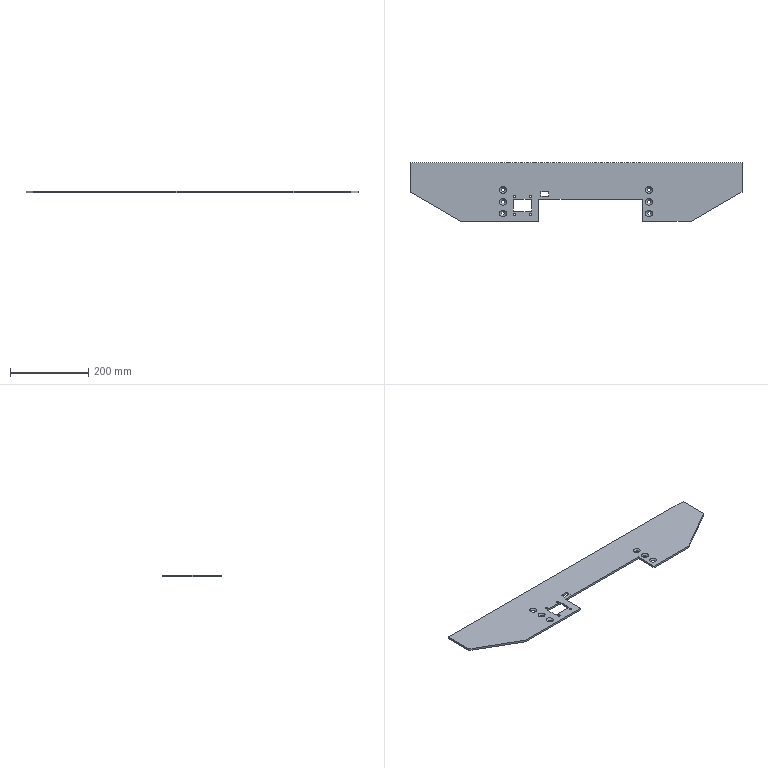Part | NX | features BREP 1 | 1 solid | 40 faces | box 850 x 150 x 5 mm | volume 499921 mm3 | plane 20 | cylinder 14 | cone 6 | commonest cylinder face diameters 9 x6 4 x4 5.2 x4
STEP:
#1=CARTESIAN_POINT('',(-114.45,17.05,0.));
#2=VERTEX_POINT('',#1);
#3=CARTESIAN_POINT('',(-117.05,17.05,0.));
#4=DIRECTION('',(0.,0.,1.));
#5=DIRECTION('',(1.,0.,0.));
#6=AXIS2_PLACEMENT_3D('',#3,#4,#5);
#7=CIRCLE('',#6,2.6);
#8=EDGE_CURVE('',#2,#2,#7,.T.);
#9=ORIENTED_EDGE('',*,*,#8,.T.);
#10=EDGE_LOOP('',(#9));
#11=FACE_BOUND('',#10,.T.);
#12=CARTESIAN_POINT('',(-114.45,17.05,-5.));
#13=VERTEX_POINT('',#12);
#14=CARTESIAN_POINT('',(-117.05,17.05,-5.));
#15=DIRECTION('',(0.,0.,1.));
#16=DIRECTION('',(1.,0.,0.));
#17=AXIS2_PLACEMENT_3D('',#14,#15,#16);
#18=CIRCLE('',#17,2.6);
#19=EDGE_CURVE('',#13,#13,#18,.T.);
#20=ORIENTED_EDGE('',*,*,#19,.F.);
#21=EDGE_LOOP('',(#20));
#22=FACE_BOUND('',#21,.T.);
#23=CARTESIAN_POINT('',(-117.05,17.05,0.));
#24=DIRECTION('',(0.,0.,1.));
#25=DIRECTION('',(1.,0.,0.));
#26=AXIS2_PLACEMENT_3D('',#23,#24,#25);
#27=CYLINDRICAL_SURFACE('',#26,2.6);
#28=ADVANCED_FACE('',(#11,#22),#27,.F.);
#29=CARTESIAN_POINT('',(-114.45,63.05,0.));
#30=VERTEX_POINT('',#29);
#31=CARTESIAN_POINT('',(-117.05,63.05,0.));
#32=DIRECTION('',(0.,0.,1.));
#33=DIRECTION('',(1.,0.,0.));
#34=AXIS2_PLACEMENT_3D('',#31,#32,#33);
#35=CIRCLE('',#34,2.6);
#36=EDGE_CURVE('',#30,#30,#35,.T.);
#37=ORIENTED_EDGE('',*,*,#36,.T.);
#38=EDGE_LOOP('',(#37));
#39=FACE_BOUND('',#38,.T.);
#40=CARTESIAN_POINT('',(-114.45,63.05,-5.));
#41=VERTEX_POINT('',#40);
#42=CARTESIAN_POINT('',(-117.05,63.05,-5.));
#43=DIRECTION('',(0.,0.,1.));
#44=DIRECTION('',(1.,0.,0.));
#45=AXIS2_PLACEMENT_3D('',#42,#43,#44);
#46=CIRCLE('',#45,2.6);
#47=EDGE_CURVE('',#41,#41,#46,.T.);
#48=ORIENTED_EDGE('',*,*,#47,.F.);
#49=EDGE_LOOP('',(#48));
#50=FACE_BOUND('',#49,.T.);
#51=CARTESIAN_POINT('',(-117.05,63.05,0.));
#52=DIRECTION('',(0.,0.,1.));
#53=DIRECTION('',(1.,0.,0.));
#54=AXIS2_PLACEMENT_3D('',#51,#52,#53);
#55=CYLINDRICAL_SURFACE('',#54,2.6);
#56=ADVANCED_FACE('',(#39,#50),#55,.F.);
#57=CARTESIAN_POINT('',(-154.45,63.05,0.));
#58=VERTEX_POINT('',#57);
#59=CARTESIAN_POINT('',(-157.05,63.05,0.));
#60=DIRECTION('',(0.,0.,1.));
#61=DIRECTION('',(1.,0.,0.));
#62=AXIS2_PLACEMENT_3D('',#59,#60,#61);
#63=CIRCLE('',#62,2.6);
#64=EDGE_CURVE('',#58,#58,#63,.T.);
#65=ORIENTED_EDGE('',*,*,#64,.T.);
#66=EDGE_LOOP('',(#65));
#67=FACE_BOUND('',#66,.T.);
#68=CARTESIAN_POINT('',(-154.45,63.05,-5.));
#69=VERTEX_POINT('',#68);
#70=CARTESIAN_POINT('',(-157.05,63.05,-5.));
#71=DIRECTION('',(0.,0.,1.));
#72=DIRECTION('',(1.,0.,0.));
#73=AXIS2_PLACEMENT_3D('',#70,#71,#72);
#74=CIRCLE('',#73,2.6);
#75=EDGE_CURVE('',#69,#69,#74,.T.);
#76=ORIENTED_EDGE('',*,*,#75,.F.);
#77=EDGE_LOOP('',(#76));
#78=FACE_BOUND('',#77,.T.);
#79=CARTESIAN_POINT('',(-157.05,63.05,0.));
#80=DIRECTION('',(0.,0.,1.));
#81=DIRECTION('',(1.,0.,0.));
#82=AXIS2_PLACEMENT_3D('',#79,#80,#81);
#83=CYLINDRICAL_SURFACE('',#82,2.6);
#84=ADVANCED_FACE('',(#67,#78),#83,.F.);
#85=CARTESIAN_POINT('',(-154.45,17.05,0.));
#86=VERTEX_POINT('',#85);
#87=CARTESIAN_POINT('',(-157.05,17.05,0.));
#88=DIRECTION('',(0.,0.,1.));
#89=DIRECTION('',(1.,0.,0.));
#90=AXIS2_PLACEMENT_3D('',#87,#88,#89);
#91=CIRCLE('',#90,2.6);
#92=EDGE_CURVE('',#86,#86,#91,.T.);
#93=ORIENTED_EDGE('',*,*,#92,.T.);
#94=EDGE_LOOP('',(#93));
#95=FACE_BOUND('',#94,.T.);
#96=CARTESIAN_POINT('',(-154.45,17.05,-5.));
#97=VERTEX_POINT('',#96);
#98=CARTESIAN_POINT('',(-157.05,17.05,-5.));
#99=DIRECTION('',(0.,0.,1.));
#100=DIRECTION('',(1.,0.,0.));
#101=AXIS2_PLACEMENT_3D('',#98,#99,#100);
#102=CIRCLE('',#101,2.6);
#103=EDGE_CURVE('',#97,#97,#102,.T.);
#104=ORIENTED_EDGE('',*,*,#103,.F.);
#105=EDGE_LOOP('',(#104));
#106=FACE_BOUND('',#105,.T.);
#107=CARTESIAN_POINT('',(-157.05,17.05,0.));
#108=DIRECTION('',(0.,0.,1.));
#109=DIRECTION('',(1.,0.,0.));
#110=AXIS2_PLACEMENT_3D('',#107,#108,#109);
#111=CYLINDRICAL_SURFACE('',#110,2.6);
#112=ADVANCED_FACE('',(#95,#106),#111,.F.);
#113=CARTESIAN_POINT('',(-178.2,20.,0.));
#114=VERTEX_POINT('',#113);
#115=CARTESIAN_POINT('',(-187.,20.,0.));
#116=DIRECTION('',(0.,0.,1.));
#117=DIRECTION('',(1.,0.,0.));
#118=AXIS2_PLACEMENT_3D('',#115,#116,#117);
#119=CIRCLE('',#118,8.8);
#120=EDGE_CURVE('',#114,#114,#119,.T.);
#121=ORIENTED_EDGE('',*,*,#120,.T.);
#122=EDGE_LOOP('',(#121));
#123=FACE_BOUND('',#122,.T.);
#124=CARTESIAN_POINT('',(-182.5,20.,-4.3));
#125=VERTEX_POINT('',#124);
#126=CARTESIAN_POINT('',(-187.,20.,-4.3));
#127=DIRECTION('',(0.,0.,1.));
#128=DIRECTION('',(1.,0.,0.));
#129=AXIS2_PLACEMENT_3D('',#126,#127,#128);
#130=CIRCLE('',#129,4.5);
#131=EDGE_CURVE('',#125,#125,#130,.T.);
#132=ORIENTED_EDGE('',*,*,#131,.F.);
#133=EDGE_LOOP('',(#132));
#134=FACE_BOUND('',#133,.T.);
#135=CARTESIAN_POINT('',(-187.,20.,0.));
#136=DIRECTION('',(0.,0.,1.));
#137=DIRECTION('',(1.,0.,0.));
#138=AXIS2_PLACEMENT_3D('',#135,#136,#137);
#139=CONICAL_SURFACE('',#138,8.8,0.7854);
#140=ADVANCED_FACE('',(#123,#134),#139,.F.);
#141=ORIENTED_EDGE('',*,*,#131,.T.);
#142=EDGE_LOOP('',(#141));
#143=FACE_BOUND('',#142,.T.);
#144=CARTESIAN_POINT('',(-182.5,20.,-5.));
#145=VERTEX_POINT('',#144);
#146=CARTESIAN_POINT('',(-187.,20.,-5.));
#147=DIRECTION('',(0.,0.,1.));
#148=DIRECTION('',(1.,0.,0.));
#149=AXIS2_PLACEMENT_3D('',#146,#147,#148);
#150=CIRCLE('',#149,4.5);
#151=EDGE_CURVE('',#145,#145,#150,.T.);
#152=ORIENTED_EDGE('',*,*,#151,.F.);
#153=EDGE_LOOP('',(#152));
#154=FACE_BOUND('',#153,.T.);
#155=CARTESIAN_POINT('',(-187.,20.,0.));
#156=DIRECTION('',(0.,0.,1.));
#157=DIRECTION('',(1.,0.,0.));
#158=AXIS2_PLACEMENT_3D('',#155,#156,#157);
#159=CYLINDRICAL_SURFACE('',#158,4.5);
#160=ADVANCED_FACE('',(#143,#154),#159,.F.);
#161=CARTESIAN_POINT('',(-178.2,50.,0.));
#162=VERTEX_POINT('',#161);
#163=CARTESIAN_POINT('',(-187.,50.,0.));
#164=DIRECTION('',(0.,0.,1.));
#165=DIRECTION('',(1.,0.,0.));
#166=AXIS2_PLACEMENT_3D('',#163,#164,#165);
#167=CIRCLE('',#166,8.8);
#168=EDGE_CURVE('',#162,#162,#167,.T.);
#169=ORIENTED_EDGE('',*,*,#168,.T.);
#170=EDGE_LOOP('',(#169));
#171=FACE_BOUND('',#170,.T.);
#172=CARTESIAN_POINT('',(-182.5,50.,-4.3));
#173=VERTEX_POINT('',#172);
#174=CARTESIAN_POINT('',(-187.,50.,-4.3));
#175=DIRECTION('',(0.,0.,1.));
#176=DIRECTION('',(1.,0.,0.));
#177=AXIS2_PLACEMENT_3D('',#174,#175,#176);
#178=CIRCLE('',#177,4.5);
#179=EDGE_CURVE('',#173,#173,#178,.T.);
#180=ORIENTED_EDGE('',*,*,#179,.F.);
#181=EDGE_LOOP('',(#180));
#182=FACE_BOUND('',#181,.T.);
#183=CARTESIAN_POINT('',(-187.,50.,0.));
#184=DIRECTION('',(0.,0.,1.));
#185=DIRECTION('',(1.,0.,0.));
#186=AXIS2_PLACEMENT_3D('',#183,#184,#185);
#187=CONICAL_SURFACE('',#186,8.8,0.7854);
#188=ADVANCED_FACE('',(#171,#182),#187,.F.);
#189=ORIENTED_EDGE('',*,*,#179,.T.);
#190=EDGE_LOOP('',(#189));
#191=FACE_BOUND('',#190,.T.);
#192=CARTESIAN_POINT('',(-182.5,50.,-5.));
#193=VERTEX_POINT('',#192);
#194=CARTESIAN_POINT('',(-187.,50.,-5.));
#195=DIRECTION('',(0.,0.,1.));
#196=DIRECTION('',(1.,0.,0.));
#197=AXIS2_PLACEMENT_3D('',#194,#195,#196);
#198=CIRCLE('',#197,4.5);
#199=EDGE_CURVE('',#193,#193,#198,.T.);
#200=ORIENTED_EDGE('',*,*,#199,.F.);
#201=EDGE_LOOP('',(#200));
#202=FACE_BOUND('',#201,.T.);
#203=CARTESIAN_POINT('',(-187.,50.,0.));
#204=DIRECTION('',(0.,0.,1.));
#205=DIRECTION('',(1.,0.,0.));
#206=AXIS2_PLACEMENT_3D('',#203,#204,#205);
#207=CYLINDRICAL_SURFACE('',#206,4.5);
#208=ADVANCED_FACE('',(#191,#202),#207,.F.);
#209=CARTESIAN_POINT('',(-178.2,80.,0.));
#210=VERTEX_POINT('',#209);
#211=CARTESIAN_POINT('',(-187.,80.,0.));
#212=DIRECTION('',(0.,0.,1.));
#213=DIRECTION('',(1.,0.,0.));
#214=AXIS2_PLACEMENT_3D('',#211,#212,#213);
#215=CIRCLE('',#214,8.8);
#216=EDGE_CURVE('',#210,#210,#215,.T.);
#217=ORIENTED_EDGE('',*,*,#216,.T.);
#218=EDGE_LOOP('',(#217));
#219=FACE_BOUND('',#218,.T.);
#220=CARTESIAN_POINT('',(-182.5,80.,-4.3));
#221=VERTEX_POINT('',#220);
#222=CARTESIAN_POINT('',(-187.,80.,-4.3));
#223=DIRECTION('',(0.,0.,1.));
#224=DIRECTION('',(1.,0.,0.));
#225=AXIS2_PLACEMENT_3D('',#222,#223,#224);
#226=CIRCLE('',#225,4.5);
#227=EDGE_CURVE('',#221,#221,#226,.T.);
#228=ORIENTED_EDGE('',*,*,#227,.F.);
#229=EDGE_LOOP('',(#228));
#230=FACE_BOUND('',#229,.T.);
#231=CARTESIAN_POINT('',(-187.,80.,0.));
#232=DIRECTION('',(0.,0.,1.));
#233=DIRECTION('',(1.,0.,0.));
#234=AXIS2_PLACEMENT_3D('',#231,#232,#233);
#235=CONICAL_SURFACE('',#234,8.8,0.7854);
#236=ADVANCED_FACE('',(#219,#230),#235,.F.);
#237=ORIENTED_EDGE('',*,*,#227,.T.);
#238=EDGE_LOOP('',(#237));
#239=FACE_BOUND('',#238,.T.);
#240=CARTESIAN_POINT('',(-182.5,80.,-5.));
#241=VERTEX_POINT('',#240);
#242=CARTESIAN_POINT('',(-187.,80.,-5.));
#243=DIRECTION('',(0.,0.,1.));
#244=DIRECTION('',(1.,0.,0.));
#245=AXIS2_PLACEMENT_3D('',#242,#243,#244);
#246=CIRCLE('',#245,4.5);
#247=EDGE_CURVE('',#241,#241,#246,.T.);
#248=ORIENTED_EDGE('',*,*,#247,.F.);
#249=EDGE_LOOP('',(#248));
#250=FACE_BOUND('',#249,.T.);
#251=CARTESIAN_POINT('',(-187.,80.,0.));
#252=DIRECTION('',(0.,0.,1.));
#253=DIRECTION('',(1.,0.,0.));
#254=AXIS2_PLACEMENT_3D('',#251,#252,#253);
#255=CYLINDRICAL_SURFACE('',#254,4.5);
#256=ADVANCED_FACE('',(#239,#250),#255,.F.);
#257=CARTESIAN_POINT('',(195.8,80.,0.));
#258=VERTEX_POINT('',#257);
#259=CARTESIAN_POINT('',(187.,80.,0.));
#260=DIRECTION('',(0.,0.,1.));
#261=DIRECTION('',(1.,0.,0.));
#262=AXIS2_PLACEMENT_3D('',#259,#260,#261);
#263=CIRCLE('',#262,8.8);
#264=EDGE_CURVE('',#258,#258,#263,.T.);
#265=ORIENTED_EDGE('',*,*,#264,.T.);
#266=EDGE_LOOP('',(#265));
#267=FACE_BOUND('',#266,.T.);
#268=CARTESIAN_POINT('',(191.5,80.,-4.3));
#269=VERTEX_POINT('',#268);
#270=CARTESIAN_POINT('',(187.,80.,-4.3));
#271=DIRECTION('',(0.,0.,1.));
#272=DIRECTION('',(1.,0.,0.));
#273=AXIS2_PLACEMENT_3D('',#270,#271,#272);
#274=CIRCLE('',#273,4.5);
#275=EDGE_CURVE('',#269,#269,#274,.T.);
#276=ORIENTED_EDGE('',*,*,#275,.F.);
#277=EDGE_LOOP('',(#276));
#278=FACE_BOUND('',#277,.T.);
#279=CARTESIAN_POINT('',(187.,80.,0.));
#280=DIRECTION('',(0.,0.,1.));
#281=DIRECTION('',(1.,0.,0.));
#282=AXIS2_PLACEMENT_3D('',#279,#280,#281);
#283=CONICAL_SURFACE('',#282,8.8,0.7854);
#284=ADVANCED_FACE('',(#267,#278),#283,.F.);
#285=ORIENTED_EDGE('',*,*,#275,.T.);
#286=EDGE_LOOP('',(#285));
#287=FACE_BOUND('',#286,.T.);
#288=CARTESIAN_POINT('',(191.5,80.,-5.));
#289=VERTEX_POINT('',#288);
#290=CARTESIAN_POINT('',(187.,80.,-5.));
#291=DIRECTION('',(0.,0.,1.));
#292=DIRECTION('',(1.,0.,0.));
#293=AXIS2_PLACEMENT_3D('',#290,#291,#292);
#294=CIRCLE('',#293,4.5);
#295=EDGE_CURVE('',#289,#289,#294,.T.);
#296=ORIENTED_EDGE('',*,*,#295,.F.);
#297=EDGE_LOOP('',(#296));
#298=FACE_BOUND('',#297,.T.);
#299=CARTESIAN_POINT('',(187.,80.,0.));
#300=DIRECTION('',(0.,0.,1.));
#301=DIRECTION('',(1.,0.,0.));
#302=AXIS2_PLACEMENT_3D('',#299,#300,#301);
#303=CYLINDRICAL_SURFACE('',#302,4.5);
#304=ADVANCED_FACE('',(#287,#298),#303,.F.);
#305=CARTESIAN_POINT('',(195.8,50.,0.));
#306=VERTEX_POINT('',#305);
#307=CARTESIAN_POINT('',(187.,50.,0.));
#308=DIRECTION('',(0.,0.,1.));
#309=DIRECTION('',(1.,0.,0.));
#310=AXIS2_PLACEMENT_3D('',#307,#308,#309);
#311=CIRCLE('',#310,8.8);
#312=EDGE_CURVE('',#306,#306,#311,.T.);
#313=ORIENTED_EDGE('',*,*,#312,.T.);
#314=EDGE_LOOP('',(#313));
#315=FACE_BOUND('',#314,.T.);
#316=CARTESIAN_POINT('',(191.5,50.,-4.3));
#317=VERTEX_POINT('',#316);
#318=CARTESIAN_POINT('',(187.,50.,-4.3));
#319=DIRECTION('',(0.,0.,1.));
#320=DIRECTION('',(1.,0.,0.));
#321=AXIS2_PLACEMENT_3D('',#318,#319,#320);
#322=CIRCLE('',#321,4.5);
#323=EDGE_CURVE('',#317,#317,#322,.T.);
#324=ORIENTED_EDGE('',*,*,#323,.F.);
#325=EDGE_LOOP('',(#324));
#326=FACE_BOUND('',#325,.T.);
#327=CARTESIAN_POINT('',(187.,50.,0.));
#328=DIRECTION('',(0.,0.,1.));
#329=DIRECTION('',(1.,0.,0.));
#330=AXIS2_PLACEMENT_3D('',#327,#328,#329);
#331=CONICAL_SURFACE('',#330,8.8,0.7854);
#332=ADVANCED_FACE('',(#315,#326),#331,.F.);
#333=ORIENTED_EDGE('',*,*,#323,.T.);
#334=EDGE_LOOP('',(#333));
#335=FACE_BOUND('',#334,.T.);
#336=CARTESIAN_POINT('',(191.5,50.,-5.));
#337=VERTEX_POINT('',#336);
#338=CARTESIAN_POINT('',(187.,50.,-5.));
#339=DIRECTION('',(0.,0.,1.));
#340=DIRECTION('',(1.,0.,0.));
#341=AXIS2_PLACEMENT_3D('',#338,#339,#340);
#342=CIRCLE('',#341,4.5);
#343=EDGE_CURVE('',#337,#337,#342,.T.);
#344=ORIENTED_EDGE('',*,*,#343,.F.);
#345=EDGE_LOOP('',(#344));
#346=FACE_BOUND('',#345,.T.);
#347=CARTESIAN_POINT('',(187.,50.,0.));
#348=DIRECTION('',(0.,0.,1.));
#349=DIRECTION('',(1.,0.,0.));
#350=AXIS2_PLACEMENT_3D('',#347,#348,#349);
#351=CYLINDRICAL_SURFACE('',#350,4.5);
#352=ADVANCED_FACE('',(#335,#346),#351,.F.);
#353=CARTESIAN_POINT('',(195.8,20.,0.));
#354=VERTEX_POINT('',#353);
#355=CARTESIAN_POINT('',(187.,20.,0.));
#356=DIRECTION('',(0.,0.,1.));
#357=DIRECTION('',(1.,0.,0.));
#358=AXIS2_PLACEMENT_3D('',#355,#356,#357);
#359=CIRCLE('',#358,8.8);
#360=EDGE_CURVE('',#354,#354,#359,.T.);
#361=ORIENTED_EDGE('',*,*,#360,.T.);
#362=EDGE_LOOP('',(#361));
#363=FACE_BOUND('',#362,.T.);
#364=CARTESIAN_POINT('',(191.5,20.,-4.3));
#365=VERTEX_POINT('',#364);
#366=CARTESIAN_POINT('',(187.,20.,-4.3));
#367=DIRECTION('',(0.,0.,1.));
#368=DIRECTION('',(1.,0.,0.));
#369=AXIS2_PLACEMENT_3D('',#366,#367,#368);
#370=CIRCLE('',#369,4.5);
#371=EDGE_CURVE('',#365,#365,#370,.T.);
#372=ORIENTED_EDGE('',*,*,#371,.F.);
#373=EDGE_LOOP('',(#372));
#374=FACE_BOUND('',#373,.T.);
#375=CARTESIAN_POINT('',(187.,20.,0.));
#376=DIRECTION('',(0.,0.,1.));
#377=DIRECTION('',(1.,0.,0.));
#378=AXIS2_PLACEMENT_3D('',#375,#376,#377);
#379=CONICAL_SURFACE('',#378,8.8,0.7854);
#380=ADVANCED_FACE('',(#363,#374),#379,.F.);
#381=ORIENTED_EDGE('',*,*,#371,.T.);
#382=EDGE_LOOP('',(#381));
#383=FACE_BOUND('',#382,.T.);
#384=CARTESIAN_POINT('',(191.5,20.,-5.));
#385=VERTEX_POINT('',#384);
#386=CARTESIAN_POINT('',(187.,20.,-5.));
#387=DIRECTION('',(0.,0.,1.));
#388=DIRECTION('',(1.,0.,0.));
#389=AXIS2_PLACEMENT_3D('',#386,#387,#388);
#390=CIRCLE('',#389,4.5);
#391=EDGE_CURVE('',#385,#385,#390,.T.);
#392=ORIENTED_EDGE('',*,*,#391,.F.);
#393=EDGE_LOOP('',(#392));
#394=FACE_BOUND('',#393,.T.);
#395=CARTESIAN_POINT('',(187.,20.,0.));
#396=DIRECTION('',(0.,0.,1.));
#397=DIRECTION('',(1.,0.,0.));
#398=AXIS2_PLACEMENT_3D('',#395,#396,#397);
#399=CYLINDRICAL_SURFACE('',#398,4.5);
#400=ADVANCED_FACE('',(#383,#394),#399,.F.);
#401=CARTESIAN_POINT('',(170.,0.,-5.));
#402=VERTEX_POINT('',#401);
#403=CARTESIAN_POINT('',(170.,0.,0.));
#404=VERTEX_POINT('',#403);
#405=CARTESIAN_POINT('',(170.,0.,-5.));
#406=DIRECTION('',(0.,0.,1.));
#407=VECTOR('',#406,1000.);
#408=LINE('',#405,#407);
#409=EDGE_CURVE('',#402,#404,#408,.T.);
#410=ORIENTED_EDGE('',*,*,#409,.F.);
#411=CARTESIAN_POINT('',(295.,0.,-5.));
#412=VERTEX_POINT('',#411);
#413=CARTESIAN_POINT('',(-295.,0.,-5.));
#414=DIRECTION('',(1.,0.,0.));
#415=VECTOR('',#414,1000.);
#416=LINE('',#413,#415);
#417=EDGE_CURVE('',#402,#412,#416,.T.);
#418=ORIENTED_EDGE('',*,*,#417,.T.);
#419=CARTESIAN_POINT('',(295.,0.,0.));
#420=VERTEX_POINT('',#419);
#421=CARTESIAN_POINT('',(295.,0.,-5.));
#422=DIRECTION('',(0.,0.,1.));
#423=VECTOR('',#422,1000.);
#424=LINE('',#421,#423);
#425=EDGE_CURVE('',#412,#420,#424,.T.);
#426=ORIENTED_EDGE('',*,*,#425,.T.);
#427=CARTESIAN_POINT('',(-295.,0.,0.));
#428=DIRECTION('',(1.,0.,0.));
#429=VECTOR('',#428,1000.);
#430=LINE('',#427,#429);
#431=EDGE_CURVE('',#404,#420,#430,.T.);
#432=ORIENTED_EDGE('',*,*,#431,.F.);
#433=EDGE_LOOP('',(#410,#418,#426,#432));
#434=FACE_BOUND('',#433,.T.);
#435=CARTESIAN_POINT('',(-295.,0.,-5.));
#436=DIRECTION('',(0.,-1.,0.));
#437=DIRECTION('',(1.,0.,0.));
#438=AXIS2_PLACEMENT_3D('',#435,#436,#437);
#439=PLANE('',#438);
#440=ADVANCED_FACE('',(#434),#439,.T.);
#441=CARTESIAN_POINT('',(425.,75.,0.));
#442=VERTEX_POINT('',#441);
#443=CARTESIAN_POINT('',(425.,75.,0.));
#444=DIRECTION('',(0.8662,0.4997,0.));
#445=VECTOR('',#444,1000.);
#446=LINE('',#443,#445);
#447=EDGE_CURVE('',#420,#442,#446,.T.);
#448=ORIENTED_EDGE('',*,*,#447,.F.);
#449=ORIENTED_EDGE('',*,*,#425,.F.);
#450=CARTESIAN_POINT('',(425.,75.,-5.));
#451=VERTEX_POINT('',#450);
#452=CARTESIAN_POINT('',(425.,75.,-5.));
#453=DIRECTION('',(0.8662,0.4997,0.));
#454=VECTOR('',#453,1000.);
#455=LINE('',#452,#454);
#456=EDGE_CURVE('',#412,#451,#455,.T.);
#457=ORIENTED_EDGE('',*,*,#456,.T.);
#458=CARTESIAN_POINT('',(425.,75.,-5.));
#459=DIRECTION('',(0.,0.,1.));
#460=VECTOR('',#459,1000.);
#461=LINE('',#458,#460);
#462=EDGE_CURVE('',#451,#442,#461,.T.);
#463=ORIENTED_EDGE('',*,*,#462,.T.);
#464=EDGE_LOOP('',(#448,#449,#457,#463));
#465=FACE_BOUND('',#464,.T.);
#466=CARTESIAN_POINT('',(425.,75.,-5.));
#467=DIRECTION('',(0.4997,-0.8662,0.));
#468=DIRECTION('',(0.8662,0.4997,0.));
#469=AXIS2_PLACEMENT_3D('',#466,#467,#468);
#470=PLANE('',#469);
#471=ADVANCED_FACE('',(#465),#470,.T.);
#472=CARTESIAN_POINT('',(-95.,0.,0.));
#473=VERTEX_POINT('',#472);
#474=CARTESIAN_POINT('',(-95.,0.,-5.));
#475=VERTEX_POINT('',#474);
#476=CARTESIAN_POINT('',(-95.,0.,-5.));
#477=DIRECTION('',(0.,0.,-1.));
#478=VECTOR('',#477,1000.);
#479=LINE('',#476,#478);
#480=EDGE_CURVE('',#473,#475,#479,.T.);
#481=ORIENTED_EDGE('',*,*,#480,.F.);
#482=CARTESIAN_POINT('',(-295.,0.,0.));
#483=VERTEX_POINT('',#482);
#484=CARTESIAN_POINT('',(-295.,0.,0.));
#485=DIRECTION('',(1.,0.,0.));
#486=VECTOR('',#485,1000.);
#487=LINE('',#484,#486);
#488=EDGE_CURVE('',#483,#473,#487,.T.);
#489=ORIENTED_EDGE('',*,*,#488,.F.);
#490=CARTESIAN_POINT('',(-295.,0.,-5.));
#491=VERTEX_POINT('',#490);
#492=CARTESIAN_POINT('',(-295.,0.,-5.));
#493=DIRECTION('',(0.,0.,1.));
#494=VECTOR('',#493,1000.);
#495=LINE('',#492,#494);
#496=EDGE_CURVE('',#491,#483,#495,.T.);
#497=ORIENTED_EDGE('',*,*,#496,.F.);
#498=CARTESIAN_POINT('',(-295.,0.,-5.));
#499=DIRECTION('',(1.,0.,0.));
#500=VECTOR('',#499,1000.);
#501=LINE('',#498,#500);
#502=EDGE_CURVE('',#491,#475,#501,.T.);
#503=ORIENTED_EDGE('',*,*,#502,.T.);
#504=EDGE_LOOP('',(#481,#489,#497,#503));
#505=FACE_BOUND('',#504,.T.);
#506=CARTESIAN_POINT('',(-295.,0.,-5.));
#507=DIRECTION('',(0.,-1.,0.));
#508=DIRECTION('',(1.,0.,0.));
#509=AXIS2_PLACEMENT_3D('',#506,#507,#508);
#510=PLANE('',#509);
#511=ADVANCED_FACE('',(#505),#510,.T.);
#512=CARTESIAN_POINT('',(-425.,75.,0.));
#513=VERTEX_POINT('',#512);
#514=CARTESIAN_POINT('',(-425.,75.,0.));
#515=DIRECTION('',(0.8662,-0.4997,0.));
#516=VECTOR('',#515,1000.);
#517=LINE('',#514,#516);
#518=EDGE_CURVE('',#513,#483,#517,.T.);
#519=ORIENTED_EDGE('',*,*,#518,.F.);
#520=CARTESIAN_POINT('',(-425.,75.,-5.));
#521=VERTEX_POINT('',#520);
#522=CARTESIAN_POINT('',(-425.,75.,-5.));
#523=DIRECTION('',(0.,0.,1.));
#524=VECTOR('',#523,1000.);
#525=LINE('',#522,#524);
#526=EDGE_CURVE('',#521,#513,#525,.T.);
#527=ORIENTED_EDGE('',*,*,#526,.F.);
#528=CARTESIAN_POINT('',(-425.,75.,-5.));
#529=DIRECTION('',(0.8662,-0.4997,0.));
#530=VECTOR('',#529,1000.);
#531=LINE('',#528,#530);
#532=EDGE_CURVE('',#521,#491,#531,.T.);
#533=ORIENTED_EDGE('',*,*,#532,.T.);
#534=ORIENTED_EDGE('',*,*,#496,.T.);
#535=EDGE_LOOP('',(#519,#527,#533,#534));
#536=FACE_BOUND('',#535,.T.);
#537=CARTESIAN_POINT('',(-425.,75.,-5.));
#538=DIRECTION('',(-0.4997,-0.8662,0.));
#539=DIRECTION('',(0.8662,-0.4997,0.));
#540=AXIS2_PLACEMENT_3D('',#537,#538,#539);
#541=PLANE('',#540);
#542=ADVANCED_FACE('',(#536),#541,.T.);
#543=CARTESIAN_POINT('',(-425.,150.,0.));
#544=VERTEX_POINT('',#543);
#545=CARTESIAN_POINT('',(-425.,150.,0.));
#546=DIRECTION('',(0.,-1.,0.));
#547=VECTOR('',#546,1000.);
#548=LINE('',#545,#547);
#549=EDGE_CURVE('',#544,#513,#548,.T.);
#550=ORIENTED_EDGE('',*,*,#549,.F.);
#551=CARTESIAN_POINT('',(-425.,150.,-5.));
#552=VERTEX_POINT('',#551);
#553=CARTESIAN_POINT('',(-425.,150.,-5.));
#554=DIRECTION('',(0.,0.,1.));
#555=VECTOR('',#554,1000.);
#556=LINE('',#553,#555);
#557=EDGE_CURVE('',#552,#544,#556,.T.);
#558=ORIENTED_EDGE('',*,*,#557,.F.);
#559=CARTESIAN_POINT('',(-425.,150.,-5.));
#560=DIRECTION('',(0.,-1.,0.));
#561=VECTOR('',#560,1000.);
#562=LINE('',#559,#561);
#563=EDGE_CURVE('',#552,#521,#562,.T.);
#564=ORIENTED_EDGE('',*,*,#563,.T.);
#565=ORIENTED_EDGE('',*,*,#526,.T.);
#566=EDGE_LOOP('',(#550,#558,#564,#565));
#567=FACE_BOUND('',#566,.T.);
#568=CARTESIAN_POINT('',(-425.,150.,-5.));
#569=DIRECTION('',(-1.,0.,0.));
#570=DIRECTION('',(0.,-1.,0.));
#571=AXIS2_PLACEMENT_3D('',#568,#569,#570);
#572=PLANE('',#571);
#573=ADVANCED_FACE('',(#567),#572,.T.);
#574=CARTESIAN_POINT('',(425.,150.,0.));
#575=VERTEX_POINT('',#574);
#576=CARTESIAN_POINT('',(-425.,150.,0.));
#577=DIRECTION('',(-1.,0.,0.));
#578=VECTOR('',#577,1000.);
#579=LINE('',#576,#578);
#580=EDGE_CURVE('',#575,#544,#579,.T.);
#581=ORIENTED_EDGE('',*,*,#580,.F.);
#582=CARTESIAN_POINT('',(425.,150.,-5.));
#583=VERTEX_POINT('',#582);
#584=CARTESIAN_POINT('',(425.,150.,-5.));
#585=DIRECTION('',(0.,0.,1.));
#586=VECTOR('',#585,1000.);
#587=LINE('',#584,#586);
#588=EDGE_CURVE('',#583,#575,#587,.T.);
#589=ORIENTED_EDGE('',*,*,#588,.F.);
#590=CARTESIAN_POINT('',(-425.,150.,-5.));
#591=DIRECTION('',(-1.,0.,0.));
#592=VECTOR('',#591,1000.);
#593=LINE('',#590,#592);
#594=EDGE_CURVE('',#583,#552,#593,.T.);
#595=ORIENTED_EDGE('',*,*,#594,.T.);
#596=ORIENTED_EDGE('',*,*,#557,.T.);
#597=EDGE_LOOP('',(#581,#589,#595,#596));
#598=FACE_BOUND('',#597,.T.);
#599=CARTESIAN_POINT('',(-425.,150.,-5.));
#600=DIRECTION('',(0.,1.,0.));
#601=DIRECTION('',(-1.,0.,0.));
#602=AXIS2_PLACEMENT_3D('',#599,#600,#601);
#603=PLANE('',#602);
#604=ADVANCED_FACE('',(#598),#603,.T.);
#605=CARTESIAN_POINT('',(425.,150.,0.));
#606=DIRECTION('',(0.,1.,0.));
#607=VECTOR('',#606,1000.);
#608=LINE('',#605,#607);
#609=EDGE_CURVE('',#442,#575,#608,.T.);
#610=ORIENTED_EDGE('',*,*,#609,.F.);
#611=ORIENTED_EDGE('',*,*,#462,.F.);
#612=CARTESIAN_POINT('',(425.,150.,-5.));
#613=DIRECTION('',(0.,1.,0.));
#614=VECTOR('',#613,1000.);
#615=LINE('',#612,#614);
#616=EDGE_CURVE('',#451,#583,#615,.T.);
#617=ORIENTED_EDGE('',*,*,#616,.T.);
#618=ORIENTED_EDGE('',*,*,#588,.T.);
#619=EDGE_LOOP('',(#610,#611,#617,#618));
#620=FACE_BOUND('',#619,.T.);
#621=CARTESIAN_POINT('',(425.,150.,-5.));
#622=DIRECTION('',(1.,0.,0.));
#623=DIRECTION('',(0.,1.,0.));
#624=AXIS2_PLACEMENT_3D('',#621,#622,#623);
#625=PLANE('',#624);
#626=ADVANCED_FACE('',(#620),#625,.T.);
#627=CARTESIAN_POINT('',(-69.85,76.,-5.));
#628=VERTEX_POINT('',#627);
#629=CARTESIAN_POINT('',(-89.85,76.,-5.));
#630=VERTEX_POINT('',#629);
#631=CARTESIAN_POINT('',(0.,76.,-5.));
#632=DIRECTION('',(-1.,0.,0.));
#633=VECTOR('',#632,1000.);
#634=LINE('',#631,#633);
#635=EDGE_CURVE('',#628,#630,#634,.T.);
#636=ORIENTED_EDGE('',*,*,#635,.T.);
#637=CARTESIAN_POINT('',(-89.85,64.,-5.));
#638=VERTEX_POINT('',#637);
#639=CARTESIAN_POINT('',(-89.85,0.,-5.));
#640=DIRECTION('',(0.,-1.,0.));
#641=VECTOR('',#640,1000.);
#642=LINE('',#639,#641);
#643=EDGE_CURVE('',#630,#638,#642,.T.);
#644=ORIENTED_EDGE('',*,*,#643,.T.);
#645=CARTESIAN_POINT('',(-69.85,64.,-5.));
#646=VERTEX_POINT('',#645);
#647=CARTESIAN_POINT('',(0.,64.,-5.));
#648=DIRECTION('',(1.,0.,0.));
#649=VECTOR('',#648,1000.);
#650=LINE('',#647,#649);
#651=EDGE_CURVE('',#638,#646,#650,.T.);
#652=ORIENTED_EDGE('',*,*,#651,.T.);
#653=CARTESIAN_POINT('',(-69.85,0.,-5.));
#654=DIRECTION('',(0.,1.,0.));
#655=VECTOR('',#654,1000.);
#656=LINE('',#653,#655);
#657=EDGE_CURVE('',#646,#628,#656,.T.);
#658=ORIENTED_EDGE('',*,*,#657,.T.);
#659=EDGE_LOOP('',(#636,#644,#652,#658));
#660=FACE_BOUND('',#659,.T.);
#661=ORIENTED_EDGE('',*,*,#19,.T.);
#662=EDGE_LOOP('',(#661));
#663=FACE_BOUND('',#662,.T.);
#664=ORIENTED_EDGE('',*,*,#47,.T.);
#665=EDGE_LOOP('',(#664));
#666=FACE_BOUND('',#665,.T.);
#667=ORIENTED_EDGE('',*,*,#75,.T.);
#668=EDGE_LOOP('',(#667));
#669=FACE_BOUND('',#668,.T.);
#670=ORIENTED_EDGE('',*,*,#103,.T.);
#671=EDGE_LOOP('',(#670));
#672=FACE_BOUND('',#671,.T.);
#673=ORIENTED_EDGE('',*,*,#151,.T.);
#674=EDGE_LOOP('',(#673));
#675=FACE_BOUND('',#674,.T.);
#676=ORIENTED_EDGE('',*,*,#199,.T.);
#677=EDGE_LOOP('',(#676));
#678=FACE_BOUND('',#677,.T.);
#679=ORIENTED_EDGE('',*,*,#247,.T.);
#680=EDGE_LOOP('',(#679));
#681=FACE_BOUND('',#680,.T.);
#682=ORIENTED_EDGE('',*,*,#295,.T.);
#683=EDGE_LOOP('',(#682));
#684=FACE_BOUND('',#683,.T.);
#685=ORIENTED_EDGE('',*,*,#343,.T.);
#686=EDGE_LOOP('',(#685));
#687=FACE_BOUND('',#686,.T.);
#688=ORIENTED_EDGE('',*,*,#391,.T.);
#689=EDGE_LOOP('',(#688));
#690=FACE_BOUND('',#689,.T.);
#691=ORIENTED_EDGE('',*,*,#417,.F.);
#692=CARTESIAN_POINT('',(170.,57.,-5.));
#693=VERTEX_POINT('',#692);
#694=CARTESIAN_POINT('',(170.,0.,-5.));
#695=DIRECTION('',(0.,1.,0.));
#696=VECTOR('',#695,1000.);
#697=LINE('',#694,#696);
#698=EDGE_CURVE('',#402,#693,#697,.T.);
#699=ORIENTED_EDGE('',*,*,#698,.T.);
#700=CARTESIAN_POINT('',(-95.,57.,-5.));
#701=VERTEX_POINT('',#700);
#702=CARTESIAN_POINT('',(0.,57.,-5.));
#703=DIRECTION('',(-1.,0.,0.));
#704=VECTOR('',#703,1000.);
#705=LINE('',#702,#704);
#706=EDGE_CURVE('',#693,#701,#705,.T.);
#707=ORIENTED_EDGE('',*,*,#706,.T.);
#708=CARTESIAN_POINT('',(-95.,0.,-5.));
#709=DIRECTION('',(0.,-1.,0.));
#710=VECTOR('',#709,1000.);
#711=LINE('',#708,#710);
#712=EDGE_CURVE('',#701,#475,#711,.T.);
#713=ORIENTED_EDGE('',*,*,#712,.T.);
#714=ORIENTED_EDGE('',*,*,#502,.F.);
#715=ORIENTED_EDGE('',*,*,#532,.F.);
#716=ORIENTED_EDGE('',*,*,#563,.F.);
#717=ORIENTED_EDGE('',*,*,#594,.F.);
#718=ORIENTED_EDGE('',*,*,#616,.F.);
#719=ORIENTED_EDGE('',*,*,#456,.F.);
#720=EDGE_LOOP('',(#691,#699,#707,#713,#714,#715,#716,#717,#718,#719));
#721=FACE_BOUND('',#720,.T.);
#722=CARTESIAN_POINT('',(-115.,56.1,-5.));
#723=VERTEX_POINT('',#722);
#724=CARTESIAN_POINT('',(-159.1,56.1,-5.));
#725=VERTEX_POINT('',#724);
#726=CARTESIAN_POINT('',(0.,56.1,-5.));
#727=DIRECTION('',(-1.,0.,0.));
#728=VECTOR('',#727,1000.);
#729=LINE('',#726,#728);
#730=EDGE_CURVE('',#723,#725,#729,.T.);
#731=ORIENTED_EDGE('',*,*,#730,.T.);
#732=CARTESIAN_POINT('',(-161.1,54.1,-5.));
#733=VERTEX_POINT('',#732);
#734=CARTESIAN_POINT('',(-159.1,54.1,-5.));
#735=DIRECTION('',(0.,0.,1.));
#736=DIRECTION('',(1.,0.,0.));
#737=AXIS2_PLACEMENT_3D('',#734,#735,#736);
#738=CIRCLE('',#737,2.);
#739=EDGE_CURVE('',#725,#733,#738,.T.);
#740=ORIENTED_EDGE('',*,*,#739,.T.);
#741=CARTESIAN_POINT('',(-161.1,26.,-5.));
#742=VERTEX_POINT('',#741);
#743=CARTESIAN_POINT('',(-161.1,0.,-5.));
#744=DIRECTION('',(0.,-1.,0.));
#745=VECTOR('',#744,1000.);
#746=LINE('',#743,#745);
#747=EDGE_CURVE('',#733,#742,#746,.T.);
#748=ORIENTED_EDGE('',*,*,#747,.T.);
#749=CARTESIAN_POINT('',(-159.1,24.,-5.));
#750=VERTEX_POINT('',#749);
#751=CARTESIAN_POINT('',(-159.1,26.,-5.));
#752=DIRECTION('',(0.,0.,1.));
#753=DIRECTION('',(1.,0.,0.));
#754=AXIS2_PLACEMENT_3D('',#751,#752,#753);
#755=CIRCLE('',#754,2.);
#756=EDGE_CURVE('',#742,#750,#755,.T.);
#757=ORIENTED_EDGE('',*,*,#756,.T.);
#758=CARTESIAN_POINT('',(-115.,24.,-5.));
#759=VERTEX_POINT('',#758);
#760=CARTESIAN_POINT('',(0.,24.,-5.));
#761=DIRECTION('',(1.,0.,0.));
#762=VECTOR('',#761,1000.);
#763=LINE('',#760,#762);
#764=EDGE_CURVE('',#750,#759,#763,.T.);
#765=ORIENTED_EDGE('',*,*,#764,.T.);
#766=CARTESIAN_POINT('',(-113.,26.,-5.));
#767=VERTEX_POINT('',#766);
#768=CARTESIAN_POINT('',(-115.,26.,-5.));
#769=DIRECTION('',(0.,0.,1.));
#770=DIRECTION('',(1.,0.,0.));
#771=AXIS2_PLACEMENT_3D('',#768,#769,#770);
#772=CIRCLE('',#771,2.);
#773=EDGE_CURVE('',#759,#767,#772,.T.);
#774=ORIENTED_EDGE('',*,*,#773,.T.);
#775=CARTESIAN_POINT('',(-113.,54.1,-5.));
#776=VERTEX_POINT('',#775);
#777=CARTESIAN_POINT('',(-113.,0.,-5.));
#778=DIRECTION('',(0.,1.,0.));
#779=VECTOR('',#778,1000.);
#780=LINE('',#777,#779);
#781=EDGE_CURVE('',#767,#776,#780,.T.);
#782=ORIENTED_EDGE('',*,*,#781,.T.);
#783=CARTESIAN_POINT('',(-115.,54.1,-5.));
#784=DIRECTION('',(0.,0.,1.));
#785=DIRECTION('',(1.,0.,0.));
#786=AXIS2_PLACEMENT_3D('',#783,#784,#785);
#787=CIRCLE('',#786,2.);
#788=EDGE_CURVE('',#776,#723,#787,.T.);
#789=ORIENTED_EDGE('',*,*,#788,.T.);
#790=EDGE_LOOP('',(#731,#740,#748,#757,#765,#774,#782,#789));
#791=FACE_BOUND('',#790,.T.);
#792=CARTESIAN_POINT('',(0.,0.,-5.));
#793=DIRECTION('',(0.,0.,1.));
#794=DIRECTION('',(1.,0.,0.));
#795=AXIS2_PLACEMENT_3D('',#792,#793,#794);
#796=PLANE('',#795);
#797=ADVANCED_FACE('',(#660,#663,#666,#669,#672,#675,#678,#681,#684,#687,#690,#721,#791),#796,.F.);
#798=CARTESIAN_POINT('',(-89.85,76.,0.));
#799=VERTEX_POINT('',#798);
#800=CARTESIAN_POINT('',(-89.85,64.,0.));
#801=VERTEX_POINT('',#800);
#802=CARTESIAN_POINT('',(-89.85,76.,0.));
#803=DIRECTION('',(0.,-1.,0.));
#804=VECTOR('',#803,1000.);
#805=LINE('',#802,#804);
#806=EDGE_CURVE('',#799,#801,#805,.T.);
#807=ORIENTED_EDGE('',*,*,#806,.F.);
#808=CARTESIAN_POINT('',(-69.85,76.,0.));
#809=VERTEX_POINT('',#808);
#810=CARTESIAN_POINT('',(-89.85,76.,0.));
#811=DIRECTION('',(-1.,0.,0.));
#812=VECTOR('',#811,1000.);
#813=LINE('',#810,#812);
#814=EDGE_CURVE('',#809,#799,#813,.T.);
#815=ORIENTED_EDGE('',*,*,#814,.F.);
#816=CARTESIAN_POINT('',(-69.85,64.,0.));
#817=VERTEX_POINT('',#816);
#818=CARTESIAN_POINT('',(-69.85,76.,0.));
#819=DIRECTION('',(0.,1.,0.));
#820=VECTOR('',#819,1000.);
#821=LINE('',#818,#820);
#822=EDGE_CURVE('',#817,#809,#821,.T.);
#823=ORIENTED_EDGE('',*,*,#822,.F.);
#824=CARTESIAN_POINT('',(-89.85,64.,0.));
#825=DIRECTION('',(1.,0.,0.));
#826=VECTOR('',#825,1000.);
#827=LINE('',#824,#826);
#828=EDGE_CURVE('',#801,#817,#827,.T.);
#829=ORIENTED_EDGE('',*,*,#828,.F.);
#830=EDGE_LOOP('',(#807,#815,#823,#829));
#831=FACE_BOUND('',#830,.T.);
#832=ORIENTED_EDGE('',*,*,#8,.F.);
#833=EDGE_LOOP('',(#832));
#834=FACE_BOUND('',#833,.T.);
#835=ORIENTED_EDGE('',*,*,#36,.F.);
#836=EDGE_LOOP('',(#835));
#837=FACE_BOUND('',#836,.T.);
#838=ORIENTED_EDGE('',*,*,#64,.F.);
#839=EDGE_LOOP('',(#838));
#840=FACE_BOUND('',#839,.T.);
#841=ORIENTED_EDGE('',*,*,#92,.F.);
#842=EDGE_LOOP('',(#841));
#843=FACE_BOUND('',#842,.T.);
#844=ORIENTED_EDGE('',*,*,#120,.F.);
#845=EDGE_LOOP('',(#844));
#846=FACE_BOUND('',#845,.T.);
#847=ORIENTED_EDGE('',*,*,#168,.F.);
#848=EDGE_LOOP('',(#847));
#849=FACE_BOUND('',#848,.T.);
#850=ORIENTED_EDGE('',*,*,#216,.F.);
#851=EDGE_LOOP('',(#850));
#852=FACE_BOUND('',#851,.T.);
#853=ORIENTED_EDGE('',*,*,#264,.F.);
#854=EDGE_LOOP('',(#853));
#855=FACE_BOUND('',#854,.T.);
#856=ORIENTED_EDGE('',*,*,#312,.F.);
#857=EDGE_LOOP('',(#856));
#858=FACE_BOUND('',#857,.T.);
#859=ORIENTED_EDGE('',*,*,#360,.F.);
#860=EDGE_LOOP('',(#859));
#861=FACE_BOUND('',#860,.T.);
#862=CARTESIAN_POINT('',(170.,57.,0.));
#863=VERTEX_POINT('',#862);
#864=CARTESIAN_POINT('',(170.,0.,0.));
#865=DIRECTION('',(0.,1.,0.));
#866=VECTOR('',#865,1000.);
#867=LINE('',#864,#866);
#868=EDGE_CURVE('',#404,#863,#867,.T.);
#869=ORIENTED_EDGE('',*,*,#868,.F.);
#870=ORIENTED_EDGE('',*,*,#431,.T.);
#871=ORIENTED_EDGE('',*,*,#447,.T.);
#872=ORIENTED_EDGE('',*,*,#609,.T.);
#873=ORIENTED_EDGE('',*,*,#580,.T.);
#874=ORIENTED_EDGE('',*,*,#549,.T.);
#875=ORIENTED_EDGE('',*,*,#518,.T.);
#876=ORIENTED_EDGE('',*,*,#488,.T.);
#877=CARTESIAN_POINT('',(-95.,57.,0.));
#878=VERTEX_POINT('',#877);
#879=CARTESIAN_POINT('',(-95.,57.,0.));
#880=DIRECTION('',(0.,-1.,0.));
#881=VECTOR('',#880,1000.);
#882=LINE('',#879,#881);
#883=EDGE_CURVE('',#878,#473,#882,.T.);
#884=ORIENTED_EDGE('',*,*,#883,.F.);
#885=CARTESIAN_POINT('',(-95.,57.,0.));
#886=DIRECTION('',(-1.,0.,0.));
#887=VECTOR('',#886,1000.);
#888=LINE('',#885,#887);
#889=EDGE_CURVE('',#863,#878,#888,.T.);
#890=ORIENTED_EDGE('',*,*,#889,.F.);
#891=EDGE_LOOP('',(#869,#870,#871,#872,#873,#874,#875,#876,#884,#890));
#892=FACE_BOUND('',#891,.T.);
#893=CARTESIAN_POINT('',(-159.1,24.,0.));
#894=VERTEX_POINT('',#893);
#895=CARTESIAN_POINT('',(-115.,24.,0.));
#896=VERTEX_POINT('',#895);
#897=CARTESIAN_POINT('',(-113.,24.,0.));
#898=DIRECTION('',(1.,0.,0.));
#899=VECTOR('',#898,1000.);
#900=LINE('',#897,#899);
#901=EDGE_CURVE('',#894,#896,#900,.T.);
#902=ORIENTED_EDGE('',*,*,#901,.F.);
#903=CARTESIAN_POINT('',(-161.1,26.,0.));
#904=VERTEX_POINT('',#903);
#905=CARTESIAN_POINT('',(-159.1,26.,0.));
#906=DIRECTION('',(0.,0.,-1.));
#907=DIRECTION('',(1.,0.,0.));
#908=AXIS2_PLACEMENT_3D('',#905,#906,#907);
#909=CIRCLE('',#908,2.);
#910=EDGE_CURVE('',#894,#904,#909,.T.);
#911=ORIENTED_EDGE('',*,*,#910,.T.);
#912=CARTESIAN_POINT('',(-161.1,54.1,0.));
#913=VERTEX_POINT('',#912);
#914=CARTESIAN_POINT('',(-161.1,56.1,0.));
#915=DIRECTION('',(0.,-1.,0.));
#916=VECTOR('',#915,1000.);
#917=LINE('',#914,#916);
#918=EDGE_CURVE('',#913,#904,#917,.T.);
#919=ORIENTED_EDGE('',*,*,#918,.F.);
#920=CARTESIAN_POINT('',(-159.1,56.1,0.));
#921=VERTEX_POINT('',#920);
#922=CARTESIAN_POINT('',(-159.1,54.1,0.));
#923=DIRECTION('',(0.,0.,-1.));
#924=DIRECTION('',(1.,0.,0.));
#925=AXIS2_PLACEMENT_3D('',#922,#923,#924);
#926=CIRCLE('',#925,2.);
#927=EDGE_CURVE('',#913,#921,#926,.T.);
#928=ORIENTED_EDGE('',*,*,#927,.T.);
#929=CARTESIAN_POINT('',(-115.,56.1,0.));
#930=VERTEX_POINT('',#929);
#931=CARTESIAN_POINT('',(-113.,56.1,0.));
#932=DIRECTION('',(-1.,0.,0.));
#933=VECTOR('',#932,1000.);
#934=LINE('',#931,#933);
#935=EDGE_CURVE('',#930,#921,#934,.T.);
#936=ORIENTED_EDGE('',*,*,#935,.F.);
#937=CARTESIAN_POINT('',(-113.,54.1,0.));
#938=VERTEX_POINT('',#937);
#939=CARTESIAN_POINT('',(-115.,54.1,0.));
#940=DIRECTION('',(0.,0.,-1.));
#941=DIRECTION('',(1.,0.,0.));
#942=AXIS2_PLACEMENT_3D('',#939,#940,#941);
#943=CIRCLE('',#942,2.);
#944=EDGE_CURVE('',#930,#938,#943,.T.);
#945=ORIENTED_EDGE('',*,*,#944,.T.);
#946=CARTESIAN_POINT('',(-113.,26.,0.));
#947=VERTEX_POINT('',#946);
#948=CARTESIAN_POINT('',(-113.,56.1,0.));
#949=DIRECTION('',(0.,1.,0.));
#950=VECTOR('',#949,1000.);
#951=LINE('',#948,#950);
#952=EDGE_CURVE('',#947,#938,#951,.T.);
#953=ORIENTED_EDGE('',*,*,#952,.F.);
#954=CARTESIAN_POINT('',(-115.,26.,0.));
#955=DIRECTION('',(0.,0.,-1.));
#956=DIRECTION('',(1.,0.,0.));
#957=AXIS2_PLACEMENT_3D('',#954,#955,#956);
#958=CIRCLE('',#957,2.);
#959=EDGE_CURVE('',#947,#896,#958,.T.);
#960=ORIENTED_EDGE('',*,*,#959,.T.);
#961=EDGE_LOOP('',(#902,#911,#919,#928,#936,#945,#953,#960));
#962=FACE_BOUND('',#961,.T.);
#963=CARTESIAN_POINT('',(0.,0.,0.));
#964=DIRECTION('',(0.,0.,1.));
#965=DIRECTION('',(1.,0.,0.));
#966=AXIS2_PLACEMENT_3D('',#963,#964,#965);
#967=PLANE('',#966);
#968=ADVANCED_FACE('',(#831,#834,#837,#840,#843,#846,#849,#852,#855,#858,#861,#892,#962),#967,.T.);
#969=ORIENTED_EDGE('',*,*,#901,.T.);
#970=CARTESIAN_POINT('',(-115.,24.,-5.));
#971=DIRECTION('',(0.,0.,-1.));
#972=VECTOR('',#971,1000.);
#973=LINE('',#970,#972);
#974=EDGE_CURVE('',#896,#759,#973,.T.);
#975=ORIENTED_EDGE('',*,*,#974,.T.);
#976=ORIENTED_EDGE('',*,*,#764,.F.);
#977=CARTESIAN_POINT('',(-159.1,24.,0.));
#978=DIRECTION('',(0.,0.,1.));
#979=VECTOR('',#978,1000.);
#980=LINE('',#977,#979);
#981=EDGE_CURVE('',#750,#894,#980,.T.);
#982=ORIENTED_EDGE('',*,*,#981,.T.);
#983=EDGE_LOOP('',(#969,#975,#976,#982));
#984=FACE_BOUND('',#983,.T.);
#985=CARTESIAN_POINT('',(-113.,24.,-10.));
#986=DIRECTION('',(0.,-1.,0.));
#987=DIRECTION('',(1.,0.,0.));
#988=AXIS2_PLACEMENT_3D('',#985,#986,#987);
#989=PLANE('',#988);
#990=ADVANCED_FACE('',(#984),#989,.F.);
#991=ORIENTED_EDGE('',*,*,#918,.T.);
#992=CARTESIAN_POINT('',(-161.1,26.,-5.));
#993=DIRECTION('',(0.,0.,-1.));
#994=VECTOR('',#993,1000.);
#995=LINE('',#992,#994);
#996=EDGE_CURVE('',#904,#742,#995,.T.);
#997=ORIENTED_EDGE('',*,*,#996,.T.);
#998=ORIENTED_EDGE('',*,*,#747,.F.);
#999=CARTESIAN_POINT('',(-161.1,54.1,0.));
#1000=DIRECTION('',(0.,0.,1.));
#1001=VECTOR('',#1000,1000.);
#1002=LINE('',#999,#1001);
#1003=EDGE_CURVE('',#733,#913,#1002,.T.);
#1004=ORIENTED_EDGE('',*,*,#1003,.T.);
#1005=EDGE_LOOP('',(#991,#997,#998,#1004));
#1006=FACE_BOUND('',#1005,.T.);
#1007=CARTESIAN_POINT('',(-161.1,56.1,-10.));
#1008=DIRECTION('',(-1.,0.,0.));
#1009=DIRECTION('',(0.,0.,1.));
#1010=AXIS2_PLACEMENT_3D('',#1007,#1008,#1009);
#1011=PLANE('',#1010);
#1012=ADVANCED_FACE('',(#1006),#1011,.F.);
#1013=ORIENTED_EDGE('',*,*,#935,.T.);
#1014=CARTESIAN_POINT('',(-159.1,56.1,-5.));
#1015=DIRECTION('',(0.,0.,-1.));
#1016=VECTOR('',#1015,1000.);
#1017=LINE('',#1014,#1016);
#1018=EDGE_CURVE('',#921,#725,#1017,.T.);
#1019=ORIENTED_EDGE('',*,*,#1018,.T.);
#1020=ORIENTED_EDGE('',*,*,#730,.F.);
#1021=CARTESIAN_POINT('',(-115.,56.1,0.));
#1022=DIRECTION('',(0.,0.,1.));
#1023=VECTOR('',#1022,1000.);
#1024=LINE('',#1021,#1023);
#1025=EDGE_CURVE('',#723,#930,#1024,.T.);
#1026=ORIENTED_EDGE('',*,*,#1025,.T.);
#1027=EDGE_LOOP('',(#1013,#1019,#1020,#1026));
#1028=FACE_BOUND('',#1027,.T.);
#1029=CARTESIAN_POINT('',(-113.,56.1,-10.));
#1030=DIRECTION('',(0.,1.,0.));
#1031=DIRECTION('',(-1.,0.,0.));
#1032=AXIS2_PLACEMENT_3D('',#1029,#1030,#1031);
#1033=PLANE('',#1032);
#1034=ADVANCED_FACE('',(#1028),#1033,.F.);
#1035=ORIENTED_EDGE('',*,*,#781,.F.);
#1036=CARTESIAN_POINT('',(-113.,26.,0.));
#1037=DIRECTION('',(0.,0.,1.));
#1038=VECTOR('',#1037,1000.);
#1039=LINE('',#1036,#1038);
#1040=EDGE_CURVE('',#767,#947,#1039,.T.);
#1041=ORIENTED_EDGE('',*,*,#1040,.T.);
#1042=ORIENTED_EDGE('',*,*,#952,.T.);
#1043=CARTESIAN_POINT('',(-113.,54.1,-5.));
#1044=DIRECTION('',(0.,0.,-1.));
#1045=VECTOR('',#1044,1000.);
#1046=LINE('',#1043,#1045);
#1047=EDGE_CURVE('',#938,#776,#1046,.T.);
#1048=ORIENTED_EDGE('',*,*,#1047,.T.);
#1049=EDGE_LOOP('',(#1035,#1041,#1042,#1048));
#1050=FACE_BOUND('',#1049,.T.);
#1051=CARTESIAN_POINT('',(-113.,56.1,-10.));
#1052=DIRECTION('',(1.,0.,0.));
#1053=DIRECTION('',(0.,0.,-1.));
#1054=AXIS2_PLACEMENT_3D('',#1051,#1052,#1053);
#1055=PLANE('',#1054);
#1056=ADVANCED_FACE('',(#1050),#1055,.F.);
#1057=CARTESIAN_POINT('',(170.,57.,-10.));
#1058=DIRECTION('',(0.,0.,1.));
#1059=VECTOR('',#1058,1000.);
#1060=LINE('',#1057,#1059);
#1061=EDGE_CURVE('',#693,#863,#1060,.T.);
#1062=ORIENTED_EDGE('',*,*,#1061,.T.);
#1063=ORIENTED_EDGE('',*,*,#889,.T.);
#1064=CARTESIAN_POINT('',(-95.,57.,-10.));
#1065=DIRECTION('',(0.,0.,1.));
#1066=VECTOR('',#1065,1000.);
#1067=LINE('',#1064,#1066);
#1068=EDGE_CURVE('',#701,#878,#1067,.T.);
#1069=ORIENTED_EDGE('',*,*,#1068,.F.);
#1070=ORIENTED_EDGE('',*,*,#706,.F.);
#1071=EDGE_LOOP('',(#1062,#1063,#1069,#1070));
#1072=FACE_BOUND('',#1071,.T.);
#1073=CARTESIAN_POINT('',(-95.,57.,-10.));
#1074=DIRECTION('',(0.,1.,0.));
#1075=DIRECTION('',(0.,0.,1.));
#1076=AXIS2_PLACEMENT_3D('',#1073,#1074,#1075);
#1077=PLANE('',#1076);
#1078=ADVANCED_FACE('',(#1072),#1077,.F.);
#1079=ORIENTED_EDGE('',*,*,#409,.T.);
#1080=ORIENTED_EDGE('',*,*,#868,.T.);
#1081=ORIENTED_EDGE('',*,*,#1061,.F.);
#1082=ORIENTED_EDGE('',*,*,#698,.F.);
#1083=EDGE_LOOP('',(#1079,#1080,#1081,#1082));
#1084=FACE_BOUND('',#1083,.T.);
#1085=CARTESIAN_POINT('',(170.,57.,-10.));
#1086=DIRECTION('',(1.,0.,0.));
#1087=DIRECTION('',(0.,0.,-1.));
#1088=AXIS2_PLACEMENT_3D('',#1085,#1086,#1087);
#1089=PLANE('',#1088);
#1090=ADVANCED_FACE('',(#1084),#1089,.F.);
#1091=ORIENTED_EDGE('',*,*,#480,.T.);
#1092=ORIENTED_EDGE('',*,*,#712,.F.);
#1093=ORIENTED_EDGE('',*,*,#1068,.T.);
#1094=ORIENTED_EDGE('',*,*,#883,.T.);
#1095=EDGE_LOOP('',(#1091,#1092,#1093,#1094));
#1096=FACE_BOUND('',#1095,.T.);
#1097=CARTESIAN_POINT('',(-95.,57.,-10.));
#1098=DIRECTION('',(-1.,0.,0.));
#1099=DIRECTION('',(0.,0.,1.));
#1100=AXIS2_PLACEMENT_3D('',#1097,#1098,#1099);
#1101=PLANE('',#1100);
#1102=ADVANCED_FACE('',(#1096),#1101,.F.);
#1103=ORIENTED_EDGE('',*,*,#773,.F.);
#1104=ORIENTED_EDGE('',*,*,#974,.F.);
#1105=ORIENTED_EDGE('',*,*,#959,.F.);
#1106=ORIENTED_EDGE('',*,*,#1040,.F.);
#1107=EDGE_LOOP('',(#1103,#1104,#1105,#1106));
#1108=FACE_BOUND('',#1107,.T.);
#1109=CARTESIAN_POINT('',(-115.,26.,-10.));
#1110=DIRECTION('',(0.,0.,-1.));
#1111=DIRECTION('',(-1.,0.,0.));
#1112=AXIS2_PLACEMENT_3D('',#1109,#1110,#1111);
#1113=CYLINDRICAL_SURFACE('',#1112,2.);
#1114=ADVANCED_FACE('',(#1108),#1113,.F.);
#1115=ORIENTED_EDGE('',*,*,#756,.F.);
#1116=ORIENTED_EDGE('',*,*,#996,.F.);
#1117=ORIENTED_EDGE('',*,*,#910,.F.);
#1118=ORIENTED_EDGE('',*,*,#981,.F.);
#1119=EDGE_LOOP('',(#1115,#1116,#1117,#1118));
#1120=FACE_BOUND('',#1119,.T.);
#1121=CARTESIAN_POINT('',(-159.1,26.,-10.));
#1122=DIRECTION('',(0.,0.,-1.));
#1123=DIRECTION('',(-1.,0.,0.));
#1124=AXIS2_PLACEMENT_3D('',#1121,#1122,#1123);
#1125=CYLINDRICAL_SURFACE('',#1124,2.);
#1126=ADVANCED_FACE('',(#1120),#1125,.F.);
#1127=ORIENTED_EDGE('',*,*,#739,.F.);
#1128=ORIENTED_EDGE('',*,*,#1018,.F.);
#1129=ORIENTED_EDGE('',*,*,#927,.F.);
#1130=ORIENTED_EDGE('',*,*,#1003,.F.);
#1131=EDGE_LOOP('',(#1127,#1128,#1129,#1130));
#1132=FACE_BOUND('',#1131,.T.);
#1133=CARTESIAN_POINT('',(-159.1,54.1,-10.));
#1134=DIRECTION('',(0.,0.,-1.));
#1135=DIRECTION('',(-1.,0.,0.));
#1136=AXIS2_PLACEMENT_3D('',#1133,#1134,#1135);
#1137=CYLINDRICAL_SURFACE('',#1136,2.);
#1138=ADVANCED_FACE('',(#1132),#1137,.F.);
#1139=ORIENTED_EDGE('',*,*,#788,.F.);
#1140=ORIENTED_EDGE('',*,*,#1047,.F.);
#1141=ORIENTED_EDGE('',*,*,#944,.F.);
#1142=ORIENTED_EDGE('',*,*,#1025,.F.);
#1143=EDGE_LOOP('',(#1139,#1140,#1141,#1142));
#1144=FACE_BOUND('',#1143,.T.);
#1145=CARTESIAN_POINT('',(-115.,54.1,-10.));
#1146=DIRECTION('',(0.,0.,-1.));
#1147=DIRECTION('',(-1.,0.,0.));
#1148=AXIS2_PLACEMENT_3D('',#1145,#1146,#1147);
#1149=CYLINDRICAL_SURFACE('',#1148,2.);
#1150=ADVANCED_FACE('',(#1144),#1149,.F.);
#1151=CARTESIAN_POINT('',(-89.85,76.,-10.));
#1152=DIRECTION('',(0.,0.,1.));
#1153=VECTOR('',#1152,1000.);
#1154=LINE('',#1151,#1153);
#1155=EDGE_CURVE('',#630,#799,#1154,.T.);
#1156=ORIENTED_EDGE('',*,*,#1155,.T.);
#1157=ORIENTED_EDGE('',*,*,#806,.T.);
#1158=CARTESIAN_POINT('',(-89.85,64.,-10.));
#1159=DIRECTION('',(0.,0.,1.));
#1160=VECTOR('',#1159,1000.);
#1161=LINE('',#1158,#1160);
#1162=EDGE_CURVE('',#638,#801,#1161,.T.);
#1163=ORIENTED_EDGE('',*,*,#1162,.F.);
#1164=ORIENTED_EDGE('',*,*,#643,.F.);
#1165=EDGE_LOOP('',(#1156,#1157,#1163,#1164));
#1166=FACE_BOUND('',#1165,.T.);
#1167=CARTESIAN_POINT('',(-89.85,76.,-10.));
#1168=DIRECTION('',(-1.,0.,0.));
#1169=DIRECTION('',(0.,0.,1.));
#1170=AXIS2_PLACEMENT_3D('',#1167,#1168,#1169);
#1171=PLANE('',#1170);
#1172=ADVANCED_FACE('',(#1166),#1171,.F.);
#1173=CARTESIAN_POINT('',(-69.85,76.,-10.));
#1174=DIRECTION('',(0.,0.,1.));
#1175=VECTOR('',#1174,1000.);
#1176=LINE('',#1173,#1175);
#1177=EDGE_CURVE('',#628,#809,#1176,.T.);
#1178=ORIENTED_EDGE('',*,*,#1177,.T.);
#1179=ORIENTED_EDGE('',*,*,#814,.T.);
#1180=ORIENTED_EDGE('',*,*,#1155,.F.);
#1181=ORIENTED_EDGE('',*,*,#635,.F.);
#1182=EDGE_LOOP('',(#1178,#1179,#1180,#1181));
#1183=FACE_BOUND('',#1182,.T.);
#1184=CARTESIAN_POINT('',(-89.85,76.,-10.));
#1185=DIRECTION('',(0.,1.,0.));
#1186=DIRECTION('',(0.,0.,1.));
#1187=AXIS2_PLACEMENT_3D('',#1184,#1185,#1186);
#1188=PLANE('',#1187);
#1189=ADVANCED_FACE('',(#1183),#1188,.F.);
#1190=CARTESIAN_POINT('',(-69.85,64.,-10.));
#1191=DIRECTION('',(0.,0.,1.));
#1192=VECTOR('',#1191,1000.);
#1193=LINE('',#1190,#1192);
#1194=EDGE_CURVE('',#646,#817,#1193,.T.);
#1195=ORIENTED_EDGE('',*,*,#1194,.T.);
#1196=ORIENTED_EDGE('',*,*,#822,.T.);
#1197=ORIENTED_EDGE('',*,*,#1177,.F.);
#1198=ORIENTED_EDGE('',*,*,#657,.F.);
#1199=EDGE_LOOP('',(#1195,#1196,#1197,#1198));
#1200=FACE_BOUND('',#1199,.T.);
#1201=CARTESIAN_POINT('',(-69.85,76.,-10.));
#1202=DIRECTION('',(1.,0.,0.));
#1203=DIRECTION('',(0.,0.,-1.));
#1204=AXIS2_PLACEMENT_3D('',#1201,#1202,#1203);
#1205=PLANE('',#1204);
#1206=ADVANCED_FACE('',(#1200),#1205,.F.);
#1207=ORIENTED_EDGE('',*,*,#1162,.T.);
#1208=ORIENTED_EDGE('',*,*,#828,.T.);
#1209=ORIENTED_EDGE('',*,*,#1194,.F.);
#1210=ORIENTED_EDGE('',*,*,#651,.F.);
#1211=EDGE_LOOP('',(#1207,#1208,#1209,#1210));
#1212=FACE_BOUND('',#1211,.T.);
#1213=CARTESIAN_POINT('',(-89.85,64.,-10.));
#1214=DIRECTION('',(0.,-1.,0.));
#1215=DIRECTION('',(0.,0.,-1.));
#1216=AXIS2_PLACEMENT_3D('',#1213,#1214,#1215);
#1217=PLANE('',#1216);
#1218=ADVANCED_FACE('',(#1212),#1217,.F.);
#1219=CLOSED_SHELL('',(#28,#56,#84,#112,#140,#160,#188,#208,#236,#256,#284,#304,#332,#352,#380,#400,#440,#471,#511,#542,#573,#604,#626,#797,#968,#990,#1012,#1034,#1056,#1078,#1090,#1102,#1114,#1126,#1138,#1150,#1172,#1189,#1206,#1218));
#1220=MANIFOLD_SOLID_BREP('',#1219);
#1221=(LENGTH_UNIT()NAMED_UNIT(*)SI_UNIT(.MILLI.,.METRE.));
#1222=UNCERTAINTY_MEASURE_WITH_UNIT(LENGTH_MEASURE(0.00001),#1221,'','');
#1223=(NAMED_UNIT(*)PLANE_ANGLE_UNIT()SI_UNIT($,.RADIAN.));
#1224=(NAMED_UNIT(*)SI_UNIT($,.STERADIAN.)SOLID_ANGLE_UNIT());
#1225=(GEOMETRIC_REPRESENTATION_CONTEXT(3)GLOBAL_UNCERTAINTY_ASSIGNED_CONTEXT((#1222))GLOBAL_UNIT_ASSIGNED_CONTEXT((#1221,#1223,#1224))REPRESENTATION_CONTEXT('',''));
#1226=ADVANCED_BREP_SHAPE_REPRESENTATION('',(#1220),#1225);